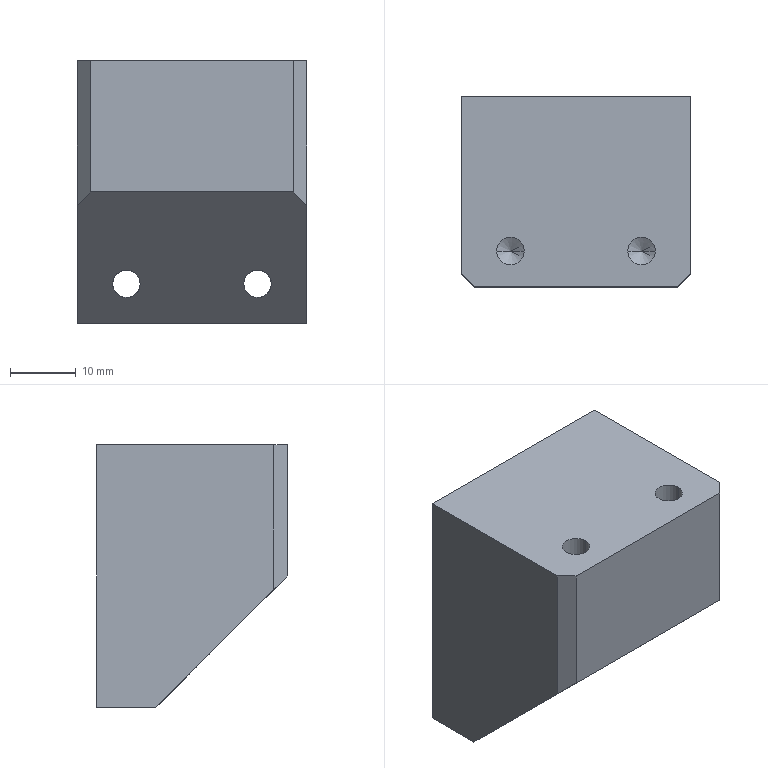Part | SolidWorks | features 3DProfileFeature 2, Chamfer 2, HoleWzd 2, Extrusion 1 | 1 solid | 21 faces | box 35 x 29 x 40 mm | volume 32746 mm3 | plane 9 | cylinder 8 | cone 4 | commonest cylinder face diameters 4.2 x8
STEP:
#1=CARTESIAN_POINT('',(-10.,11.9,-11.9));
#2=VERTEX_POINT('',#1);
#3=CARTESIAN_POINT('',(-10.,16.1,-16.1));
#4=VERTEX_POINT('',#3);
#5=CARTESIAN_POINT('',(-10.,11.9,-11.9));
#6=CARTESIAN_POINT('',(-14.2,11.9,-11.9));
#7=CARTESIAN_POINT('',(-14.2,16.1,-16.1));
#8=CARTESIAN_POINT('',(-10.,16.1,-16.1));
#9=(BOUNDED_CURVE()B_SPLINE_CURVE(3,(#5,#6,#7,#8),.UNSPECIFIED.,.F.,.T.)B_SPLINE_CURVE_WITH_KNOTS((4,4),(3.142,6.283),.UNSPECIFIED.)CURVE()GEOMETRIC_REPRESENTATION_ITEM()RATIONAL_B_SPLINE_CURVE((1.,0.3333,0.3333,1.))REPRESENTATION_ITEM(''));
#10=EDGE_CURVE('',#2,#4,#9,.T.);
#11=ORIENTED_EDGE('',*,*,#10,.T.);
#12=CARTESIAN_POINT('',(-10.,29.,-16.1));
#13=VERTEX_POINT('',#12);
#14=CARTESIAN_POINT('',(-10.,29.,-16.1));
#15=DIRECTION('',(0.,1.,0.));
#16=VECTOR('',#15,1000.);
#17=LINE('',#14,#16);
#18=EDGE_CURVE('',#4,#13,#17,.T.);
#19=ORIENTED_EDGE('',*,*,#18,.T.);
#20=CARTESIAN_POINT('',(-10.,29.,-11.9));
#21=VERTEX_POINT('',#20);
#22=CARTESIAN_POINT('',(-10.,29.,-14.));
#23=DIRECTION('',(0.,1.,0.));
#24=DIRECTION('',(0.,0.,1.));
#25=AXIS2_PLACEMENT_3D('',#22,#23,#24);
#26=CIRCLE('',#25,2.1);
#27=EDGE_CURVE('',#13,#21,#26,.T.);
#28=ORIENTED_EDGE('',*,*,#27,.T.);
#29=CARTESIAN_POINT('',(-10.,29.,-11.9));
#30=DIRECTION('',(0.,1.,0.));
#31=VECTOR('',#30,1000.);
#32=LINE('',#29,#31);
#33=EDGE_CURVE('',#2,#21,#32,.T.);
#34=ORIENTED_EDGE('',*,*,#33,.F.);
#35=EDGE_LOOP('',(#11,#19,#28,#34));
#36=FACE_OUTER_BOUND('',#35,.T.);
#37=CARTESIAN_POINT('',(-10.,29.,-14.));
#38=DIRECTION('',(0.,1.,0.));
#39=DIRECTION('',(0.,0.,1.));
#40=AXIS2_PLACEMENT_3D('',#37,#38,#39);
#41=CYLINDRICAL_SURFACE('',#40,2.1);
#42=ADVANCED_FACE('',(#36),#41,.F.);
#43=CARTESIAN_POINT('',(10.,11.9,-11.9));
#44=VERTEX_POINT('',#43);
#45=CARTESIAN_POINT('',(10.,16.1,-16.1));
#46=VERTEX_POINT('',#45);
#47=CARTESIAN_POINT('',(10.,11.9,-11.9));
#48=CARTESIAN_POINT('',(5.8,11.9,-11.9));
#49=CARTESIAN_POINT('',(5.8,16.1,-16.1));
#50=CARTESIAN_POINT('',(10.,16.1,-16.1));
#51=(BOUNDED_CURVE()B_SPLINE_CURVE(3,(#47,#48,#49,#50),.UNSPECIFIED.,.F.,.F.)B_SPLINE_CURVE_WITH_KNOTS((4,4),(3.142,6.283),.UNSPECIFIED.)CURVE()GEOMETRIC_REPRESENTATION_ITEM()RATIONAL_B_SPLINE_CURVE((1.,0.3333,0.3333,1.))REPRESENTATION_ITEM(''));
#52=EDGE_CURVE('',#44,#46,#51,.T.);
#53=ORIENTED_EDGE('',*,*,#52,.T.);
#54=CARTESIAN_POINT('',(10.,29.,-16.1));
#55=VERTEX_POINT('',#54);
#56=CARTESIAN_POINT('',(10.,29.,-16.1));
#57=DIRECTION('',(0.,1.,0.));
#58=VECTOR('',#57,1000.);
#59=LINE('',#56,#58);
#60=EDGE_CURVE('',#46,#55,#59,.T.);
#61=ORIENTED_EDGE('',*,*,#60,.T.);
#62=CARTESIAN_POINT('',(10.,29.,-11.9));
#63=VERTEX_POINT('',#62);
#64=CARTESIAN_POINT('',(10.,29.,-14.));
#65=DIRECTION('',(0.,1.,0.));
#66=DIRECTION('',(0.,0.,1.));
#67=AXIS2_PLACEMENT_3D('',#64,#65,#66);
#68=CIRCLE('',#67,2.1);
#69=EDGE_CURVE('',#55,#63,#68,.T.);
#70=ORIENTED_EDGE('',*,*,#69,.T.);
#71=CARTESIAN_POINT('',(10.,29.,-11.9));
#72=DIRECTION('',(0.,1.,0.));
#73=VECTOR('',#72,1000.);
#74=LINE('',#71,#73);
#75=EDGE_CURVE('',#44,#63,#74,.T.);
#76=ORIENTED_EDGE('',*,*,#75,.F.);
#77=EDGE_LOOP('',(#53,#61,#70,#76));
#78=FACE_OUTER_BOUND('',#77,.T.);
#79=CARTESIAN_POINT('',(10.,29.,-14.));
#80=DIRECTION('',(0.,1.,0.));
#81=DIRECTION('',(0.,0.,1.));
#82=AXIS2_PLACEMENT_3D('',#79,#80,#81);
#83=CYLINDRICAL_SURFACE('',#82,2.1);
#84=ADVANCED_FACE('',(#78),#83,.F.);
#85=CARTESIAN_POINT('',(-12.1,5.5,7.6));
#86=VERTEX_POINT('',#85);
#87=CARTESIAN_POINT('',(-7.9,5.5,7.6));
#88=VERTEX_POINT('',#87);
#89=CARTESIAN_POINT('',(-10.,5.5,7.6));
#90=DIRECTION('',(0.,0.,1.));
#91=DIRECTION('',(1.,0.,0.));
#92=AXIS2_PLACEMENT_3D('',#89,#90,#91);
#93=CIRCLE('',#92,2.1);
#94=EDGE_CURVE('',#86,#88,#93,.T.);
#95=ORIENTED_EDGE('',*,*,#94,.F.);
#96=CARTESIAN_POINT('',(-12.1,5.5,20.));
#97=VERTEX_POINT('',#96);
#98=CARTESIAN_POINT('',(-12.1,5.5,20.));
#99=DIRECTION('',(0.,0.,1.));
#100=VECTOR('',#99,1000.);
#101=LINE('',#98,#100);
#102=EDGE_CURVE('',#86,#97,#101,.T.);
#103=ORIENTED_EDGE('',*,*,#102,.T.);
#104=CARTESIAN_POINT('',(-7.9,5.5,20.));
#105=VERTEX_POINT('',#104);
#106=CARTESIAN_POINT('',(-10.,5.5,20.));
#107=DIRECTION('',(0.,0.,1.));
#108=DIRECTION('',(1.,0.,0.));
#109=AXIS2_PLACEMENT_3D('',#106,#107,#108);
#110=CIRCLE('',#109,2.1);
#111=EDGE_CURVE('',#97,#105,#110,.T.);
#112=ORIENTED_EDGE('',*,*,#111,.T.);
#113=CARTESIAN_POINT('',(-7.9,5.5,20.));
#114=DIRECTION('',(0.,0.,1.));
#115=VECTOR('',#114,1000.);
#116=LINE('',#113,#115);
#117=EDGE_CURVE('',#88,#105,#116,.T.);
#118=ORIENTED_EDGE('',*,*,#117,.F.);
#119=EDGE_LOOP('',(#95,#103,#112,#118));
#120=FACE_OUTER_BOUND('',#119,.T.);
#121=CARTESIAN_POINT('',(-10.,5.5,20.));
#122=DIRECTION('',(0.,0.,1.));
#123=DIRECTION('',(1.,0.,0.));
#124=AXIS2_PLACEMENT_3D('',#121,#122,#123);
#125=CYLINDRICAL_SURFACE('',#124,2.1);
#126=ADVANCED_FACE('',(#120),#125,.F.);
#127=CARTESIAN_POINT('',(-10.,5.5,6.338));
#128=VERTEX_POINT('',#127);
#129=CARTESIAN_POINT('',(-7.9,5.5,7.6));
#130=DIRECTION('',(0.8572,0.,0.515));
#131=VECTOR('',#130,1000.);
#132=LINE('',#129,#131);
#133=EDGE_CURVE('',#128,#88,#132,.T.);
#134=ORIENTED_EDGE('',*,*,#133,.F.);
#135=CARTESIAN_POINT('',(-12.1,5.5,7.6));
#136=DIRECTION('',(-0.8572,0.,0.515));
#137=VECTOR('',#136,1000.);
#138=LINE('',#135,#137);
#139=EDGE_CURVE('',#128,#86,#138,.T.);
#140=ORIENTED_EDGE('',*,*,#139,.T.);
#141=ORIENTED_EDGE('',*,*,#94,.T.);
#142=EDGE_LOOP('',(#134,#140,#141));
#143=FACE_OUTER_BOUND('',#142,.T.);
#144=CARTESIAN_POINT('',(-10.,5.5,7.6));
#145=DIRECTION('',(0.,0.,1.));
#146=DIRECTION('',(1.,0.,0.));
#147=AXIS2_PLACEMENT_3D('',#144,#145,#146);
#148=CONICAL_SURFACE('',#147,2.1,1.03);
#149=ADVANCED_FACE('',(#143),#148,.F.);
#150=CARTESIAN_POINT('',(7.9,5.5,7.6));
#151=VERTEX_POINT('',#150);
#152=CARTESIAN_POINT('',(12.1,5.5,7.6));
#153=VERTEX_POINT('',#152);
#154=CARTESIAN_POINT('',(10.,5.5,7.6));
#155=DIRECTION('',(0.,0.,1.));
#156=DIRECTION('',(1.,0.,0.));
#157=AXIS2_PLACEMENT_3D('',#154,#155,#156);
#158=CIRCLE('',#157,2.1);
#159=EDGE_CURVE('',#151,#153,#158,.T.);
#160=ORIENTED_EDGE('',*,*,#159,.F.);
#161=CARTESIAN_POINT('',(7.9,5.5,20.));
#162=VERTEX_POINT('',#161);
#163=CARTESIAN_POINT('',(7.9,5.5,20.));
#164=DIRECTION('',(0.,0.,1.));
#165=VECTOR('',#164,1000.);
#166=LINE('',#163,#165);
#167=EDGE_CURVE('',#151,#162,#166,.T.);
#168=ORIENTED_EDGE('',*,*,#167,.T.);
#169=CARTESIAN_POINT('',(12.1,5.5,20.));
#170=VERTEX_POINT('',#169);
#171=CARTESIAN_POINT('',(10.,5.5,20.));
#172=DIRECTION('',(0.,0.,1.));
#173=DIRECTION('',(1.,0.,0.));
#174=AXIS2_PLACEMENT_3D('',#171,#172,#173);
#175=CIRCLE('',#174,2.1);
#176=EDGE_CURVE('',#162,#170,#175,.T.);
#177=ORIENTED_EDGE('',*,*,#176,.T.);
#178=CARTESIAN_POINT('',(12.1,5.5,20.));
#179=DIRECTION('',(0.,0.,1.));
#180=VECTOR('',#179,1000.);
#181=LINE('',#178,#180);
#182=EDGE_CURVE('',#153,#170,#181,.T.);
#183=ORIENTED_EDGE('',*,*,#182,.F.);
#184=EDGE_LOOP('',(#160,#168,#177,#183));
#185=FACE_OUTER_BOUND('',#184,.T.);
#186=CARTESIAN_POINT('',(10.,5.5,20.));
#187=DIRECTION('',(0.,0.,1.));
#188=DIRECTION('',(1.,0.,0.));
#189=AXIS2_PLACEMENT_3D('',#186,#187,#188);
#190=CYLINDRICAL_SURFACE('',#189,2.1);
#191=ADVANCED_FACE('',(#185),#190,.F.);
#192=CARTESIAN_POINT('',(10.,5.5,6.338));
#193=VERTEX_POINT('',#192);
#194=CARTESIAN_POINT('',(12.1,5.5,7.6));
#195=DIRECTION('',(0.8572,0.,0.515));
#196=VECTOR('',#195,1000.);
#197=LINE('',#194,#196);
#198=EDGE_CURVE('',#193,#153,#197,.T.);
#199=ORIENTED_EDGE('',*,*,#198,.F.);
#200=CARTESIAN_POINT('',(7.9,5.5,7.6));
#201=DIRECTION('',(-0.8572,0.,0.515));
#202=VECTOR('',#201,1000.);
#203=LINE('',#200,#202);
#204=EDGE_CURVE('',#193,#151,#203,.T.);
#205=ORIENTED_EDGE('',*,*,#204,.T.);
#206=ORIENTED_EDGE('',*,*,#159,.T.);
#207=EDGE_LOOP('',(#199,#205,#206));
#208=FACE_OUTER_BOUND('',#207,.T.);
#209=CARTESIAN_POINT('',(10.,5.5,7.6));
#210=DIRECTION('',(0.,0.,1.));
#211=DIRECTION('',(1.,0.,0.));
#212=AXIS2_PLACEMENT_3D('',#209,#210,#211);
#213=CONICAL_SURFACE('',#212,2.1,1.03);
#214=ADVANCED_FACE('',(#208),#213,.F.);
#215=CARTESIAN_POINT('',(17.5,29.,20.));
#216=VERTEX_POINT('',#215);
#217=CARTESIAN_POINT('',(17.5,2.,20.));
#218=VERTEX_POINT('',#217);
#219=CARTESIAN_POINT('',(17.5,29.,20.));
#220=DIRECTION('',(0.,-1.,0.));
#221=VECTOR('',#220,1000.);
#222=LINE('',#219,#221);
#223=EDGE_CURVE('',#216,#218,#222,.T.);
#224=ORIENTED_EDGE('',*,*,#223,.T.);
#225=CARTESIAN_POINT('',(17.5,2.,-2.));
#226=VERTEX_POINT('',#225);
#227=CARTESIAN_POINT('',(17.5,2.,-20.));
#228=DIRECTION('',(0.,0.,-1.));
#229=VECTOR('',#228,1000.);
#230=LINE('',#227,#229);
#231=EDGE_CURVE('',#218,#226,#230,.T.);
#232=ORIENTED_EDGE('',*,*,#231,.T.);
#233=CARTESIAN_POINT('',(17.5,20.,-20.));
#234=VERTEX_POINT('',#233);
#235=CARTESIAN_POINT('',(17.5,20.,-20.));
#236=DIRECTION('',(0.,0.7071,-0.7071));
#237=VECTOR('',#236,1000.);
#238=LINE('',#235,#237);
#239=EDGE_CURVE('',#226,#234,#238,.T.);
#240=ORIENTED_EDGE('',*,*,#239,.T.);
#241=CARTESIAN_POINT('',(17.5,29.,-20.));
#242=VERTEX_POINT('',#241);
#243=CARTESIAN_POINT('',(17.5,29.,-20.));
#244=DIRECTION('',(0.,-1.,0.));
#245=VECTOR('',#244,1000.);
#246=LINE('',#243,#245);
#247=EDGE_CURVE('',#242,#234,#246,.T.);
#248=ORIENTED_EDGE('',*,*,#247,.F.);
#249=CARTESIAN_POINT('',(17.5,29.,-20.));
#250=DIRECTION('',(0.,0.,-1.));
#251=VECTOR('',#250,1000.);
#252=LINE('',#249,#251);
#253=EDGE_CURVE('',#216,#242,#252,.T.);
#254=ORIENTED_EDGE('',*,*,#253,.F.);
#255=EDGE_LOOP('',(#224,#232,#240,#248,#254));
#256=FACE_OUTER_BOUND('',#255,.T.);
#257=CARTESIAN_POINT('',(17.5,29.,-20.));
#258=DIRECTION('',(-1.,0.,0.));
#259=DIRECTION('',(0.,0.,1.));
#260=AXIS2_PLACEMENT_3D('',#257,#258,#259);
#261=PLANE('',#260);
#262=ADVANCED_FACE('',(#256),#261,.F.);
#263=ORIENTED_EDGE('',*,*,#247,.T.);
#264=CARTESIAN_POINT('',(-17.5,20.,-20.));
#265=VERTEX_POINT('',#264);
#266=CARTESIAN_POINT('',(-17.5,20.,-20.));
#267=DIRECTION('',(-1.,0.,0.));
#268=VECTOR('',#267,1000.);
#269=LINE('',#266,#268);
#270=EDGE_CURVE('',#234,#265,#269,.T.);
#271=ORIENTED_EDGE('',*,*,#270,.T.);
#272=CARTESIAN_POINT('',(-17.5,29.,-20.));
#273=VERTEX_POINT('',#272);
#274=CARTESIAN_POINT('',(-17.5,29.,-20.));
#275=DIRECTION('',(0.,-1.,0.));
#276=VECTOR('',#275,1000.);
#277=LINE('',#274,#276);
#278=EDGE_CURVE('',#273,#265,#277,.T.);
#279=ORIENTED_EDGE('',*,*,#278,.F.);
#280=CARTESIAN_POINT('',(-17.5,29.,-20.));
#281=DIRECTION('',(-1.,0.,0.));
#282=VECTOR('',#281,1000.);
#283=LINE('',#280,#282);
#284=EDGE_CURVE('',#242,#273,#283,.T.);
#285=ORIENTED_EDGE('',*,*,#284,.F.);
#286=EDGE_LOOP('',(#263,#271,#279,#285));
#287=FACE_OUTER_BOUND('',#286,.T.);
#288=CARTESIAN_POINT('',(-17.5,29.,-20.));
#289=DIRECTION('',(0.,0.,1.));
#290=DIRECTION('',(1.,0.,0.));
#291=AXIS2_PLACEMENT_3D('',#288,#289,#290);
#292=PLANE('',#291);
#293=ADVANCED_FACE('',(#287),#292,.F.);
#294=CARTESIAN_POINT('',(-17.5,2.,-2.));
#295=VERTEX_POINT('',#294);
#296=CARTESIAN_POINT('',(-17.5,20.,-20.));
#297=DIRECTION('',(0.,-0.7071,0.7071));
#298=VECTOR('',#297,1000.);
#299=LINE('',#296,#298);
#300=EDGE_CURVE('',#265,#295,#299,.T.);
#301=ORIENTED_EDGE('',*,*,#300,.T.);
#302=CARTESIAN_POINT('',(-17.5,2.,20.));
#303=VERTEX_POINT('',#302);
#304=CARTESIAN_POINT('',(-17.5,2.,-20.));
#305=DIRECTION('',(0.,0.,1.));
#306=VECTOR('',#305,1000.);
#307=LINE('',#304,#306);
#308=EDGE_CURVE('',#295,#303,#307,.T.);
#309=ORIENTED_EDGE('',*,*,#308,.T.);
#310=CARTESIAN_POINT('',(-17.5,29.,20.));
#311=VERTEX_POINT('',#310);
#312=CARTESIAN_POINT('',(-17.5,29.,20.));
#313=DIRECTION('',(0.,-1.,0.));
#314=VECTOR('',#313,1000.);
#315=LINE('',#312,#314);
#316=EDGE_CURVE('',#311,#303,#315,.T.);
#317=ORIENTED_EDGE('',*,*,#316,.F.);
#318=CARTESIAN_POINT('',(-17.5,29.,-20.));
#319=DIRECTION('',(0.,0.,1.));
#320=VECTOR('',#319,1000.);
#321=LINE('',#318,#320);
#322=EDGE_CURVE('',#273,#311,#321,.T.);
#323=ORIENTED_EDGE('',*,*,#322,.F.);
#324=ORIENTED_EDGE('',*,*,#278,.T.);
#325=EDGE_LOOP('',(#301,#309,#317,#323,#324));
#326=FACE_OUTER_BOUND('',#325,.T.);
#327=CARTESIAN_POINT('',(-17.5,29.,-20.));
#328=DIRECTION('',(1.,0.,0.));
#329=DIRECTION('',(0.,0.,-1.));
#330=AXIS2_PLACEMENT_3D('',#327,#328,#329);
#331=PLANE('',#330);
#332=ADVANCED_FACE('',(#326),#331,.F.);
#333=CARTESIAN_POINT('',(-10.,5.5,20.));
#334=DIRECTION('',(0.,0.,1.));
#335=DIRECTION('',(1.,0.,0.));
#336=AXIS2_PLACEMENT_3D('',#333,#334,#335);
#337=CIRCLE('',#336,2.1);
#338=EDGE_CURVE('',#105,#97,#337,.T.);
#339=ORIENTED_EDGE('',*,*,#338,.F.);
#340=ORIENTED_EDGE('',*,*,#111,.F.);
#341=EDGE_LOOP('',(#339,#340));
#342=FACE_BOUND('',#341,.T.);
#343=CARTESIAN_POINT('',(10.,5.5,20.));
#344=DIRECTION('',(0.,0.,1.));
#345=DIRECTION('',(1.,0.,0.));
#346=AXIS2_PLACEMENT_3D('',#343,#344,#345);
#347=CIRCLE('',#346,2.1);
#348=EDGE_CURVE('',#170,#162,#347,.T.);
#349=ORIENTED_EDGE('',*,*,#348,.F.);
#350=ORIENTED_EDGE('',*,*,#176,.F.);
#351=EDGE_LOOP('',(#349,#350));
#352=FACE_BOUND('',#351,.T.);
#353=ORIENTED_EDGE('',*,*,#316,.T.);
#354=CARTESIAN_POINT('',(-15.5,0.,20.));
#355=VERTEX_POINT('',#354);
#356=CARTESIAN_POINT('',(-17.5,2.,20.));
#357=DIRECTION('',(0.7071,-0.7071,0.));
#358=VECTOR('',#357,1000.);
#359=LINE('',#356,#358);
#360=EDGE_CURVE('',#303,#355,#359,.T.);
#361=ORIENTED_EDGE('',*,*,#360,.T.);
#362=CARTESIAN_POINT('',(15.5,0.,20.));
#363=VERTEX_POINT('',#362);
#364=CARTESIAN_POINT('',(-17.5,0.,20.));
#365=DIRECTION('',(1.,0.,0.));
#366=VECTOR('',#365,1000.);
#367=LINE('',#364,#366);
#368=EDGE_CURVE('',#355,#363,#367,.T.);
#369=ORIENTED_EDGE('',*,*,#368,.T.);
#370=CARTESIAN_POINT('',(17.5,2.,20.));
#371=DIRECTION('',(0.7071,0.7071,0.));
#372=VECTOR('',#371,1000.);
#373=LINE('',#370,#372);
#374=EDGE_CURVE('',#363,#218,#373,.T.);
#375=ORIENTED_EDGE('',*,*,#374,.T.);
#376=ORIENTED_EDGE('',*,*,#223,.F.);
#377=CARTESIAN_POINT('',(-17.5,29.,20.));
#378=DIRECTION('',(1.,0.,0.));
#379=VECTOR('',#378,1000.);
#380=LINE('',#377,#379);
#381=EDGE_CURVE('',#311,#216,#380,.T.);
#382=ORIENTED_EDGE('',*,*,#381,.F.);
#383=EDGE_LOOP('',(#353,#361,#369,#375,#376,#382));
#384=FACE_OUTER_BOUND('',#383,.T.);
#385=CARTESIAN_POINT('',(-17.5,29.,20.));
#386=DIRECTION('',(0.,0.,-1.));
#387=DIRECTION('',(-1.,0.,0.));
#388=AXIS2_PLACEMENT_3D('',#385,#386,#387);
#389=PLANE('',#388);
#390=ADVANCED_FACE('',(#342,#352,#384),#389,.F.);
#391=CARTESIAN_POINT('',(-10.,29.,-14.));
#392=DIRECTION('',(0.,1.,0.));
#393=DIRECTION('',(0.,0.,1.));
#394=AXIS2_PLACEMENT_3D('',#391,#392,#393);
#395=CIRCLE('',#394,2.1);
#396=EDGE_CURVE('',#21,#13,#395,.T.);
#397=ORIENTED_EDGE('',*,*,#396,.F.);
#398=ORIENTED_EDGE('',*,*,#27,.F.);
#399=EDGE_LOOP('',(#397,#398));
#400=FACE_BOUND('',#399,.T.);
#401=CARTESIAN_POINT('',(10.,29.,-14.));
#402=DIRECTION('',(0.,1.,0.));
#403=DIRECTION('',(0.,0.,1.));
#404=AXIS2_PLACEMENT_3D('',#401,#402,#403);
#405=CIRCLE('',#404,2.1);
#406=EDGE_CURVE('',#63,#55,#405,.T.);
#407=ORIENTED_EDGE('',*,*,#406,.F.);
#408=ORIENTED_EDGE('',*,*,#69,.F.);
#409=EDGE_LOOP('',(#407,#408));
#410=FACE_BOUND('',#409,.T.);
#411=ORIENTED_EDGE('',*,*,#253,.T.);
#412=ORIENTED_EDGE('',*,*,#284,.T.);
#413=ORIENTED_EDGE('',*,*,#322,.T.);
#414=ORIENTED_EDGE('',*,*,#381,.T.);
#415=EDGE_LOOP('',(#411,#412,#413,#414));
#416=FACE_OUTER_BOUND('',#415,.T.);
#417=CARTESIAN_POINT('',(0.,29.,0.));
#418=DIRECTION('',(0.,1.,0.));
#419=DIRECTION('',(0.,0.,1.));
#420=AXIS2_PLACEMENT_3D('',#417,#418,#419);
#421=PLANE('',#420);
#422=ADVANCED_FACE('',(#400,#410,#416),#421,.T.);
#423=ORIENTED_EDGE('',*,*,#368,.F.);
#424=CARTESIAN_POINT('',(-15.5,0.,0.));
#425=VERTEX_POINT('',#424);
#426=CARTESIAN_POINT('',(-15.5,0.,0.));
#427=DIRECTION('',(0.,0.,-1.));
#428=VECTOR('',#427,1000.);
#429=LINE('',#426,#428);
#430=EDGE_CURVE('',#355,#425,#429,.T.);
#431=ORIENTED_EDGE('',*,*,#430,.T.);
#432=CARTESIAN_POINT('',(15.5,0.,0.));
#433=VERTEX_POINT('',#432);
#434=CARTESIAN_POINT('',(0.,0.,0.));
#435=DIRECTION('',(1.,0.,0.));
#436=VECTOR('',#435,1000.);
#437=LINE('',#434,#436);
#438=EDGE_CURVE('',#425,#433,#437,.T.);
#439=ORIENTED_EDGE('',*,*,#438,.T.);
#440=CARTESIAN_POINT('',(15.5,0.,0.));
#441=DIRECTION('',(0.,0.,1.));
#442=VECTOR('',#441,1000.);
#443=LINE('',#440,#442);
#444=EDGE_CURVE('',#433,#363,#443,.T.);
#445=ORIENTED_EDGE('',*,*,#444,.T.);
#446=EDGE_LOOP('',(#423,#431,#439,#445));
#447=FACE_OUTER_BOUND('',#446,.T.);
#448=CARTESIAN_POINT('',(0.,0.,0.));
#449=DIRECTION('',(0.,1.,0.));
#450=DIRECTION('',(0.,0.,1.));
#451=AXIS2_PLACEMENT_3D('',#448,#449,#450);
#452=PLANE('',#451);
#453=ADVANCED_FACE('',(#447),#452,.F.);
#454=ORIENTED_EDGE('',*,*,#10,.F.);
#455=CARTESIAN_POINT('',(-10.,16.1,-16.1));
#456=CARTESIAN_POINT('',(-5.8,16.1,-16.1));
#457=CARTESIAN_POINT('',(-5.8,11.9,-11.9));
#458=CARTESIAN_POINT('',(-10.,11.9,-11.9));
#459=(BOUNDED_CURVE()B_SPLINE_CURVE(3,(#455,#456,#457,#458),.UNSPECIFIED.,.F.,.F.)B_SPLINE_CURVE_WITH_KNOTS((4,4),(0.,3.142),.UNSPECIFIED.)CURVE()GEOMETRIC_REPRESENTATION_ITEM()RATIONAL_B_SPLINE_CURVE((1.,0.3333,0.3333,1.))REPRESENTATION_ITEM(''));
#460=EDGE_CURVE('',#4,#2,#459,.T.);
#461=ORIENTED_EDGE('',*,*,#460,.F.);
#462=EDGE_LOOP('',(#454,#461));
#463=FACE_BOUND('',#462,.T.);
#464=ORIENTED_EDGE('',*,*,#52,.F.);
#465=CARTESIAN_POINT('',(10.,16.1,-16.1));
#466=CARTESIAN_POINT('',(14.2,16.1,-16.1));
#467=CARTESIAN_POINT('',(14.2,11.9,-11.9));
#468=CARTESIAN_POINT('',(10.,11.9,-11.9));
#469=(BOUNDED_CURVE()B_SPLINE_CURVE(3,(#465,#466,#467,#468),.UNSPECIFIED.,.F.,.F.)B_SPLINE_CURVE_WITH_KNOTS((4,4),(0.,3.142),.UNSPECIFIED.)CURVE()GEOMETRIC_REPRESENTATION_ITEM()RATIONAL_B_SPLINE_CURVE((1.,0.3333,0.3333,1.))REPRESENTATION_ITEM(''));
#470=EDGE_CURVE('',#46,#44,#469,.T.);
#471=ORIENTED_EDGE('',*,*,#470,.F.);
#472=EDGE_LOOP('',(#464,#471));
#473=FACE_BOUND('',#472,.T.);
#474=ORIENTED_EDGE('',*,*,#438,.F.);
#475=CARTESIAN_POINT('',(-29.5,14.,-14.));
#476=DIRECTION('',(-0.5774,0.5774,-0.5774));
#477=VECTOR('',#476,1000.);
#478=LINE('',#475,#477);
#479=EDGE_CURVE('',#425,#295,#478,.T.);
#480=ORIENTED_EDGE('',*,*,#479,.T.);
#481=ORIENTED_EDGE('',*,*,#300,.F.);
#482=ORIENTED_EDGE('',*,*,#270,.F.);
#483=ORIENTED_EDGE('',*,*,#239,.F.);
#484=CARTESIAN_POINT('',(17.833,2.333,-2.333));
#485=DIRECTION('',(-0.5774,-0.5774,0.5774));
#486=VECTOR('',#485,1000.);
#487=LINE('',#484,#486);
#488=EDGE_CURVE('',#226,#433,#487,.T.);
#489=ORIENTED_EDGE('',*,*,#488,.T.);
#490=EDGE_LOOP('',(#474,#480,#481,#482,#483,#489));
#491=FACE_OUTER_BOUND('',#490,.T.);
#492=CARTESIAN_POINT('',(-17.5,20.,-20.));
#493=DIRECTION('',(0.,0.7071,0.7071));
#494=DIRECTION('',(-1.,0.,0.));
#495=AXIS2_PLACEMENT_3D('',#492,#493,#494);
#496=PLANE('',#495);
#497=ADVANCED_FACE('',(#463,#473,#491),#496,.F.);
#498=ORIENTED_EDGE('',*,*,#204,.F.);
#499=ORIENTED_EDGE('',*,*,#198,.T.);
#500=CARTESIAN_POINT('',(10.,5.5,7.6));
#501=DIRECTION('',(0.,0.,1.));
#502=DIRECTION('',(1.,0.,0.));
#503=AXIS2_PLACEMENT_3D('',#500,#501,#502);
#504=CIRCLE('',#503,2.1);
#505=EDGE_CURVE('',#153,#151,#504,.T.);
#506=ORIENTED_EDGE('',*,*,#505,.T.);
#507=EDGE_LOOP('',(#498,#499,#506));
#508=FACE_OUTER_BOUND('',#507,.T.);
#509=CARTESIAN_POINT('',(10.,5.5,7.6));
#510=DIRECTION('',(0.,0.,1.));
#511=DIRECTION('',(1.,0.,0.));
#512=AXIS2_PLACEMENT_3D('',#509,#510,#511);
#513=CONICAL_SURFACE('',#512,2.1,1.03);
#514=ADVANCED_FACE('',(#508),#513,.F.);
#515=ORIENTED_EDGE('',*,*,#167,.F.);
#516=ORIENTED_EDGE('',*,*,#505,.F.);
#517=ORIENTED_EDGE('',*,*,#182,.T.);
#518=ORIENTED_EDGE('',*,*,#348,.T.);
#519=EDGE_LOOP('',(#515,#516,#517,#518));
#520=FACE_OUTER_BOUND('',#519,.T.);
#521=CARTESIAN_POINT('',(10.,5.5,20.));
#522=DIRECTION('',(0.,0.,1.));
#523=DIRECTION('',(1.,0.,0.));
#524=AXIS2_PLACEMENT_3D('',#521,#522,#523);
#525=CYLINDRICAL_SURFACE('',#524,2.1);
#526=ADVANCED_FACE('',(#520),#525,.F.);
#527=ORIENTED_EDGE('',*,*,#139,.F.);
#528=ORIENTED_EDGE('',*,*,#133,.T.);
#529=CARTESIAN_POINT('',(-10.,5.5,7.6));
#530=DIRECTION('',(0.,0.,1.));
#531=DIRECTION('',(1.,0.,0.));
#532=AXIS2_PLACEMENT_3D('',#529,#530,#531);
#533=CIRCLE('',#532,2.1);
#534=EDGE_CURVE('',#88,#86,#533,.T.);
#535=ORIENTED_EDGE('',*,*,#534,.T.);
#536=EDGE_LOOP('',(#527,#528,#535));
#537=FACE_OUTER_BOUND('',#536,.T.);
#538=CARTESIAN_POINT('',(-10.,5.5,7.6));
#539=DIRECTION('',(0.,0.,1.));
#540=DIRECTION('',(1.,0.,0.));
#541=AXIS2_PLACEMENT_3D('',#538,#539,#540);
#542=CONICAL_SURFACE('',#541,2.1,1.03);
#543=ADVANCED_FACE('',(#537),#542,.F.);
#544=ORIENTED_EDGE('',*,*,#102,.F.);
#545=ORIENTED_EDGE('',*,*,#534,.F.);
#546=ORIENTED_EDGE('',*,*,#117,.T.);
#547=ORIENTED_EDGE('',*,*,#338,.T.);
#548=EDGE_LOOP('',(#544,#545,#546,#547));
#549=FACE_OUTER_BOUND('',#548,.T.);
#550=CARTESIAN_POINT('',(-10.,5.5,20.));
#551=DIRECTION('',(0.,0.,1.));
#552=DIRECTION('',(1.,0.,0.));
#553=AXIS2_PLACEMENT_3D('',#550,#551,#552);
#554=CYLINDRICAL_SURFACE('',#553,2.1);
#555=ADVANCED_FACE('',(#549),#554,.F.);
#556=ORIENTED_EDGE('',*,*,#60,.F.);
#557=ORIENTED_EDGE('',*,*,#470,.T.);
#558=ORIENTED_EDGE('',*,*,#75,.T.);
#559=ORIENTED_EDGE('',*,*,#406,.T.);
#560=EDGE_LOOP('',(#556,#557,#558,#559));
#561=FACE_OUTER_BOUND('',#560,.T.);
#562=CARTESIAN_POINT('',(10.,29.,-14.));
#563=DIRECTION('',(0.,1.,0.));
#564=DIRECTION('',(0.,0.,1.));
#565=AXIS2_PLACEMENT_3D('',#562,#563,#564);
#566=CYLINDRICAL_SURFACE('',#565,2.1);
#567=ADVANCED_FACE('',(#561),#566,.F.);
#568=ORIENTED_EDGE('',*,*,#18,.F.);
#569=ORIENTED_EDGE('',*,*,#460,.T.);
#570=ORIENTED_EDGE('',*,*,#33,.T.);
#571=ORIENTED_EDGE('',*,*,#396,.T.);
#572=EDGE_LOOP('',(#568,#569,#570,#571));
#573=FACE_OUTER_BOUND('',#572,.T.);
#574=CARTESIAN_POINT('',(-10.,29.,-14.));
#575=DIRECTION('',(0.,1.,0.));
#576=DIRECTION('',(0.,0.,1.));
#577=AXIS2_PLACEMENT_3D('',#574,#575,#576);
#578=CYLINDRICAL_SURFACE('',#577,2.1);
#579=ADVANCED_FACE('',(#573),#578,.F.);
#580=ORIENTED_EDGE('',*,*,#479,.F.);
#581=ORIENTED_EDGE('',*,*,#430,.F.);
#582=ORIENTED_EDGE('',*,*,#360,.F.);
#583=ORIENTED_EDGE('',*,*,#308,.F.);
#584=EDGE_LOOP('',(#580,#581,#582,#583));
#585=FACE_OUTER_BOUND('',#584,.T.);
#586=CARTESIAN_POINT('',(-17.5,2.,-20.));
#587=DIRECTION('',(0.7071,0.7071,0.));
#588=DIRECTION('',(0.,0.,1.));
#589=AXIS2_PLACEMENT_3D('',#586,#587,#588);
#590=PLANE('',#589);
#591=ADVANCED_FACE('',(#585),#590,.F.);
#592=ORIENTED_EDGE('',*,*,#374,.F.);
#593=ORIENTED_EDGE('',*,*,#444,.F.);
#594=ORIENTED_EDGE('',*,*,#488,.F.);
#595=ORIENTED_EDGE('',*,*,#231,.F.);
#596=EDGE_LOOP('',(#592,#593,#594,#595));
#597=FACE_OUTER_BOUND('',#596,.T.);
#598=CARTESIAN_POINT('',(17.5,2.,-20.));
#599=DIRECTION('',(-0.7071,0.7071,0.));
#600=DIRECTION('',(0.,0.,-1.));
#601=AXIS2_PLACEMENT_3D('',#598,#599,#600);
#602=PLANE('',#601);
#603=ADVANCED_FACE('',(#597),#602,.F.);
#604=CLOSED_SHELL('',(#42,#84,#126,#149,#191,#214,#262,#293,#332,#390,#422,#453,#497,#514,#526,#543,#555,#567,#579,#591,#603));
#605=MANIFOLD_SOLID_BREP('',#604);
#606=CARTESIAN_POINT('',(0.,0.,0.));
#607=DIRECTION('',(0.,0.,1.));
#608=DIRECTION('',(1.,0.,0.));
#609=AXIS2_PLACEMENT_3D('',#606,#607,#608);
#610=(LENGTH_UNIT()NAMED_UNIT(*)SI_UNIT(.MILLI.,.METRE.));
#611=UNCERTAINTY_MEASURE_WITH_UNIT(LENGTH_MEASURE(0.00001),#610,'','');
#612=(NAMED_UNIT(*)PLANE_ANGLE_UNIT()SI_UNIT($,.RADIAN.));
#613=(NAMED_UNIT(*)SI_UNIT($,.STERADIAN.)SOLID_ANGLE_UNIT());
#614=(GEOMETRIC_REPRESENTATION_CONTEXT(3)GLOBAL_UNCERTAINTY_ASSIGNED_CONTEXT((#611))GLOBAL_UNIT_ASSIGNED_CONTEXT((#610,#612,#613))REPRESENTATION_CONTEXT('',''));
#615=ADVANCED_BREP_SHAPE_REPRESENTATION('',(#605,#609),#614);